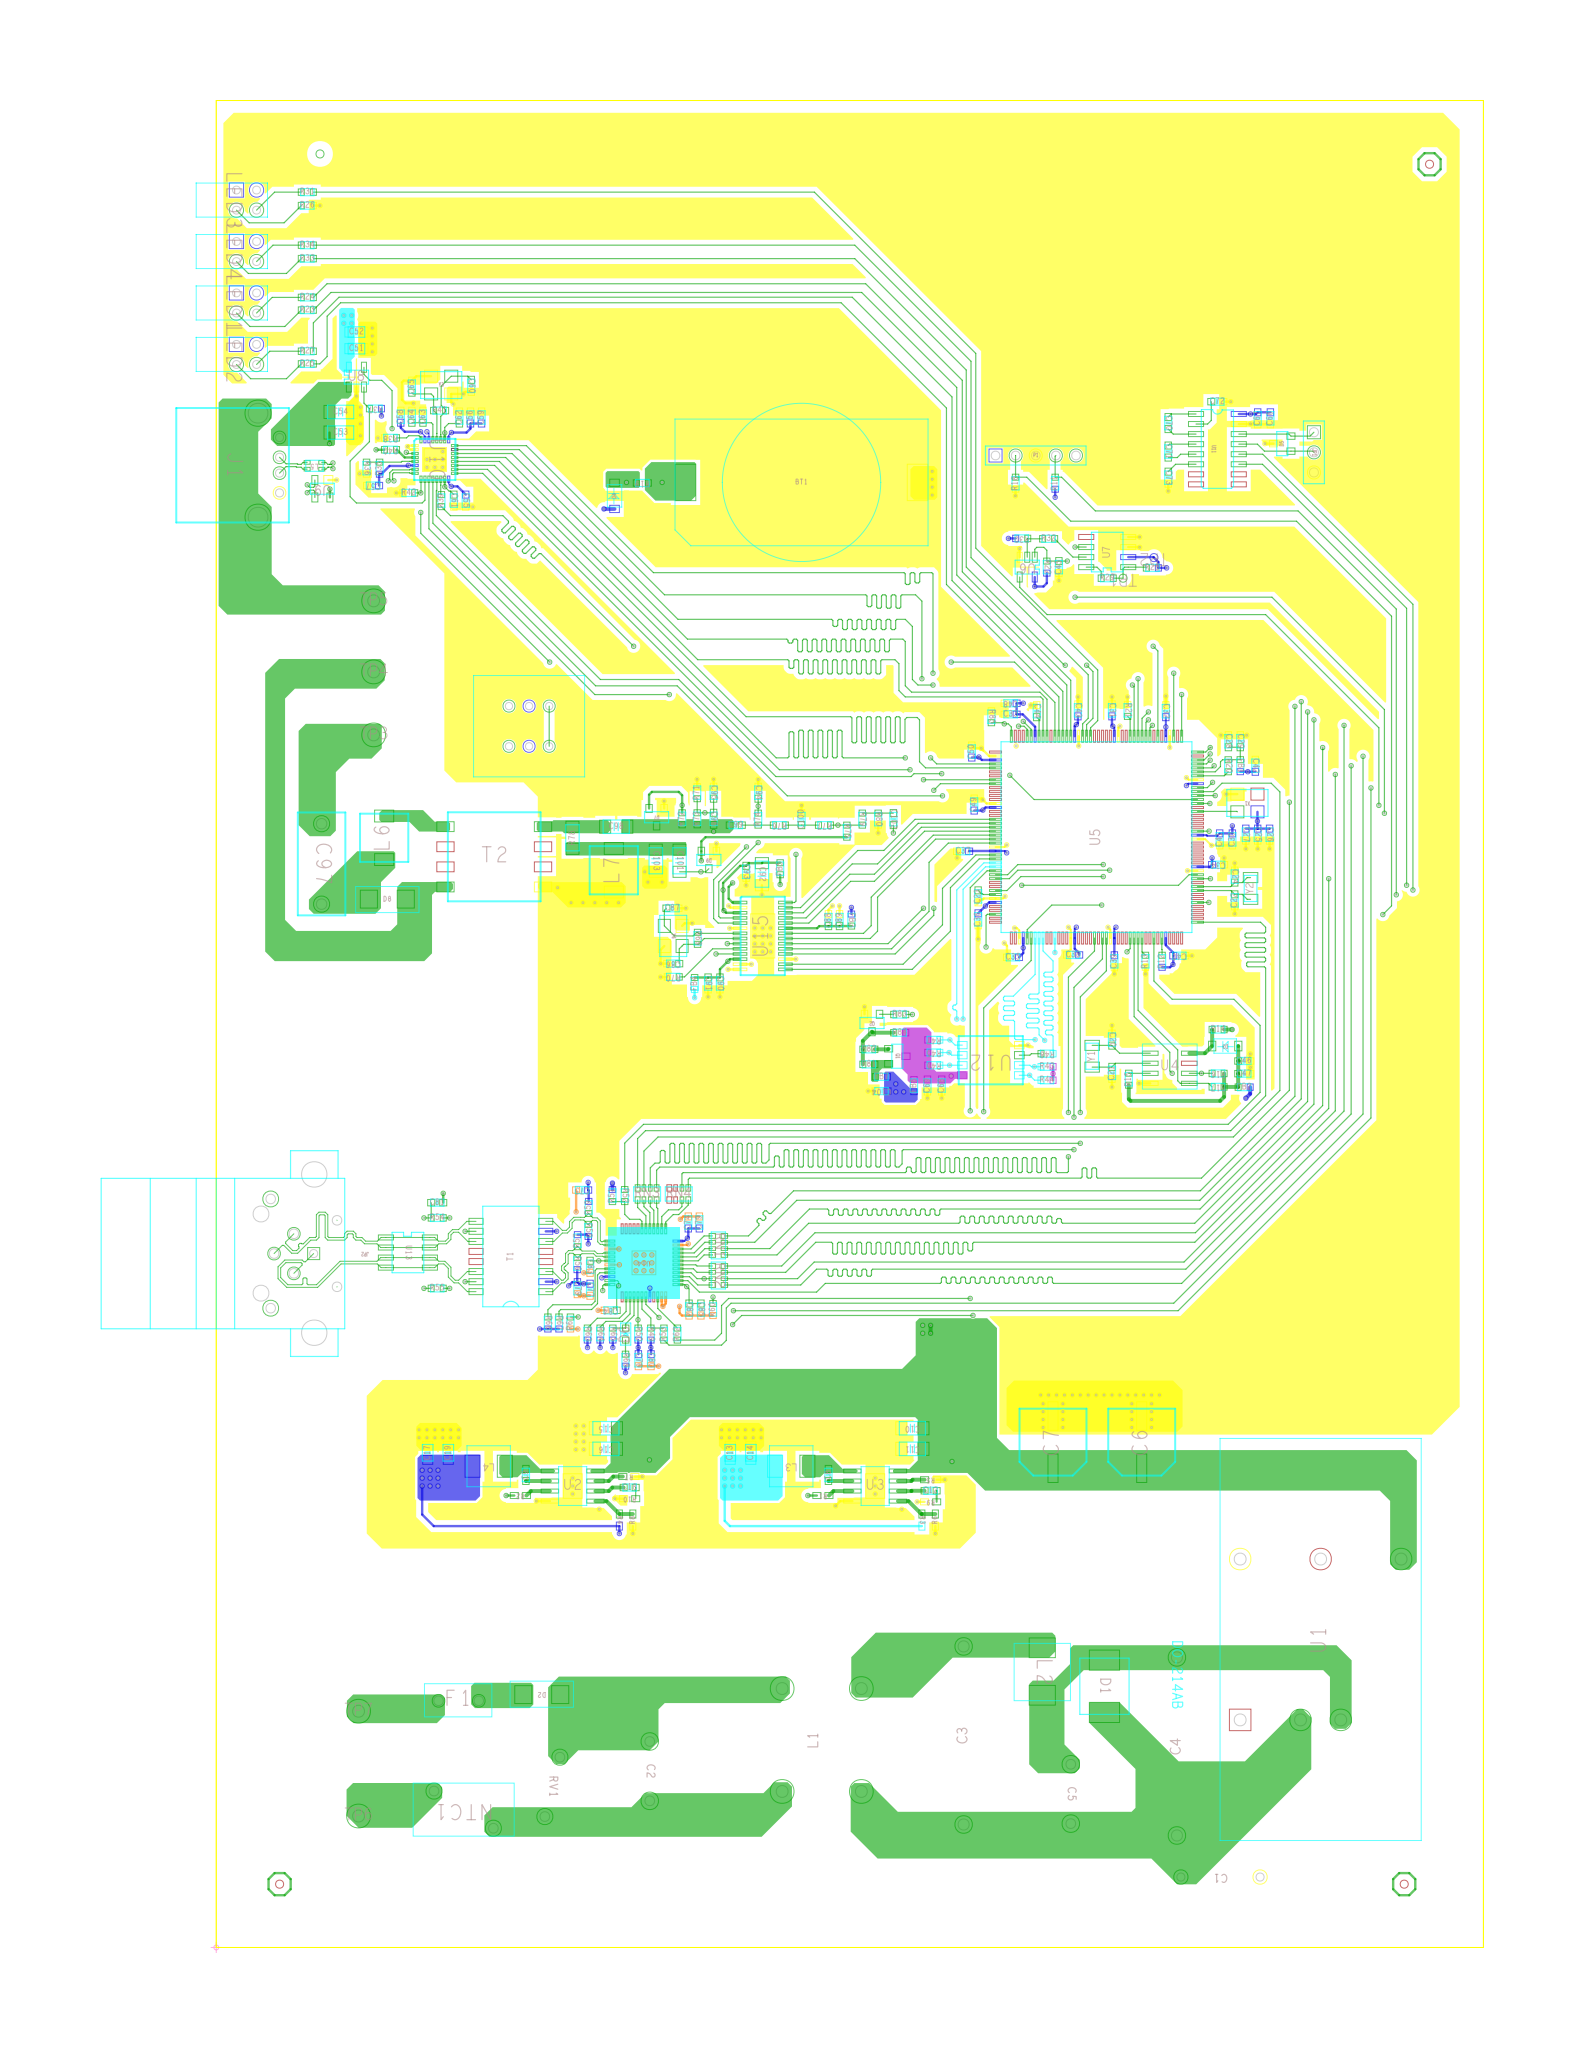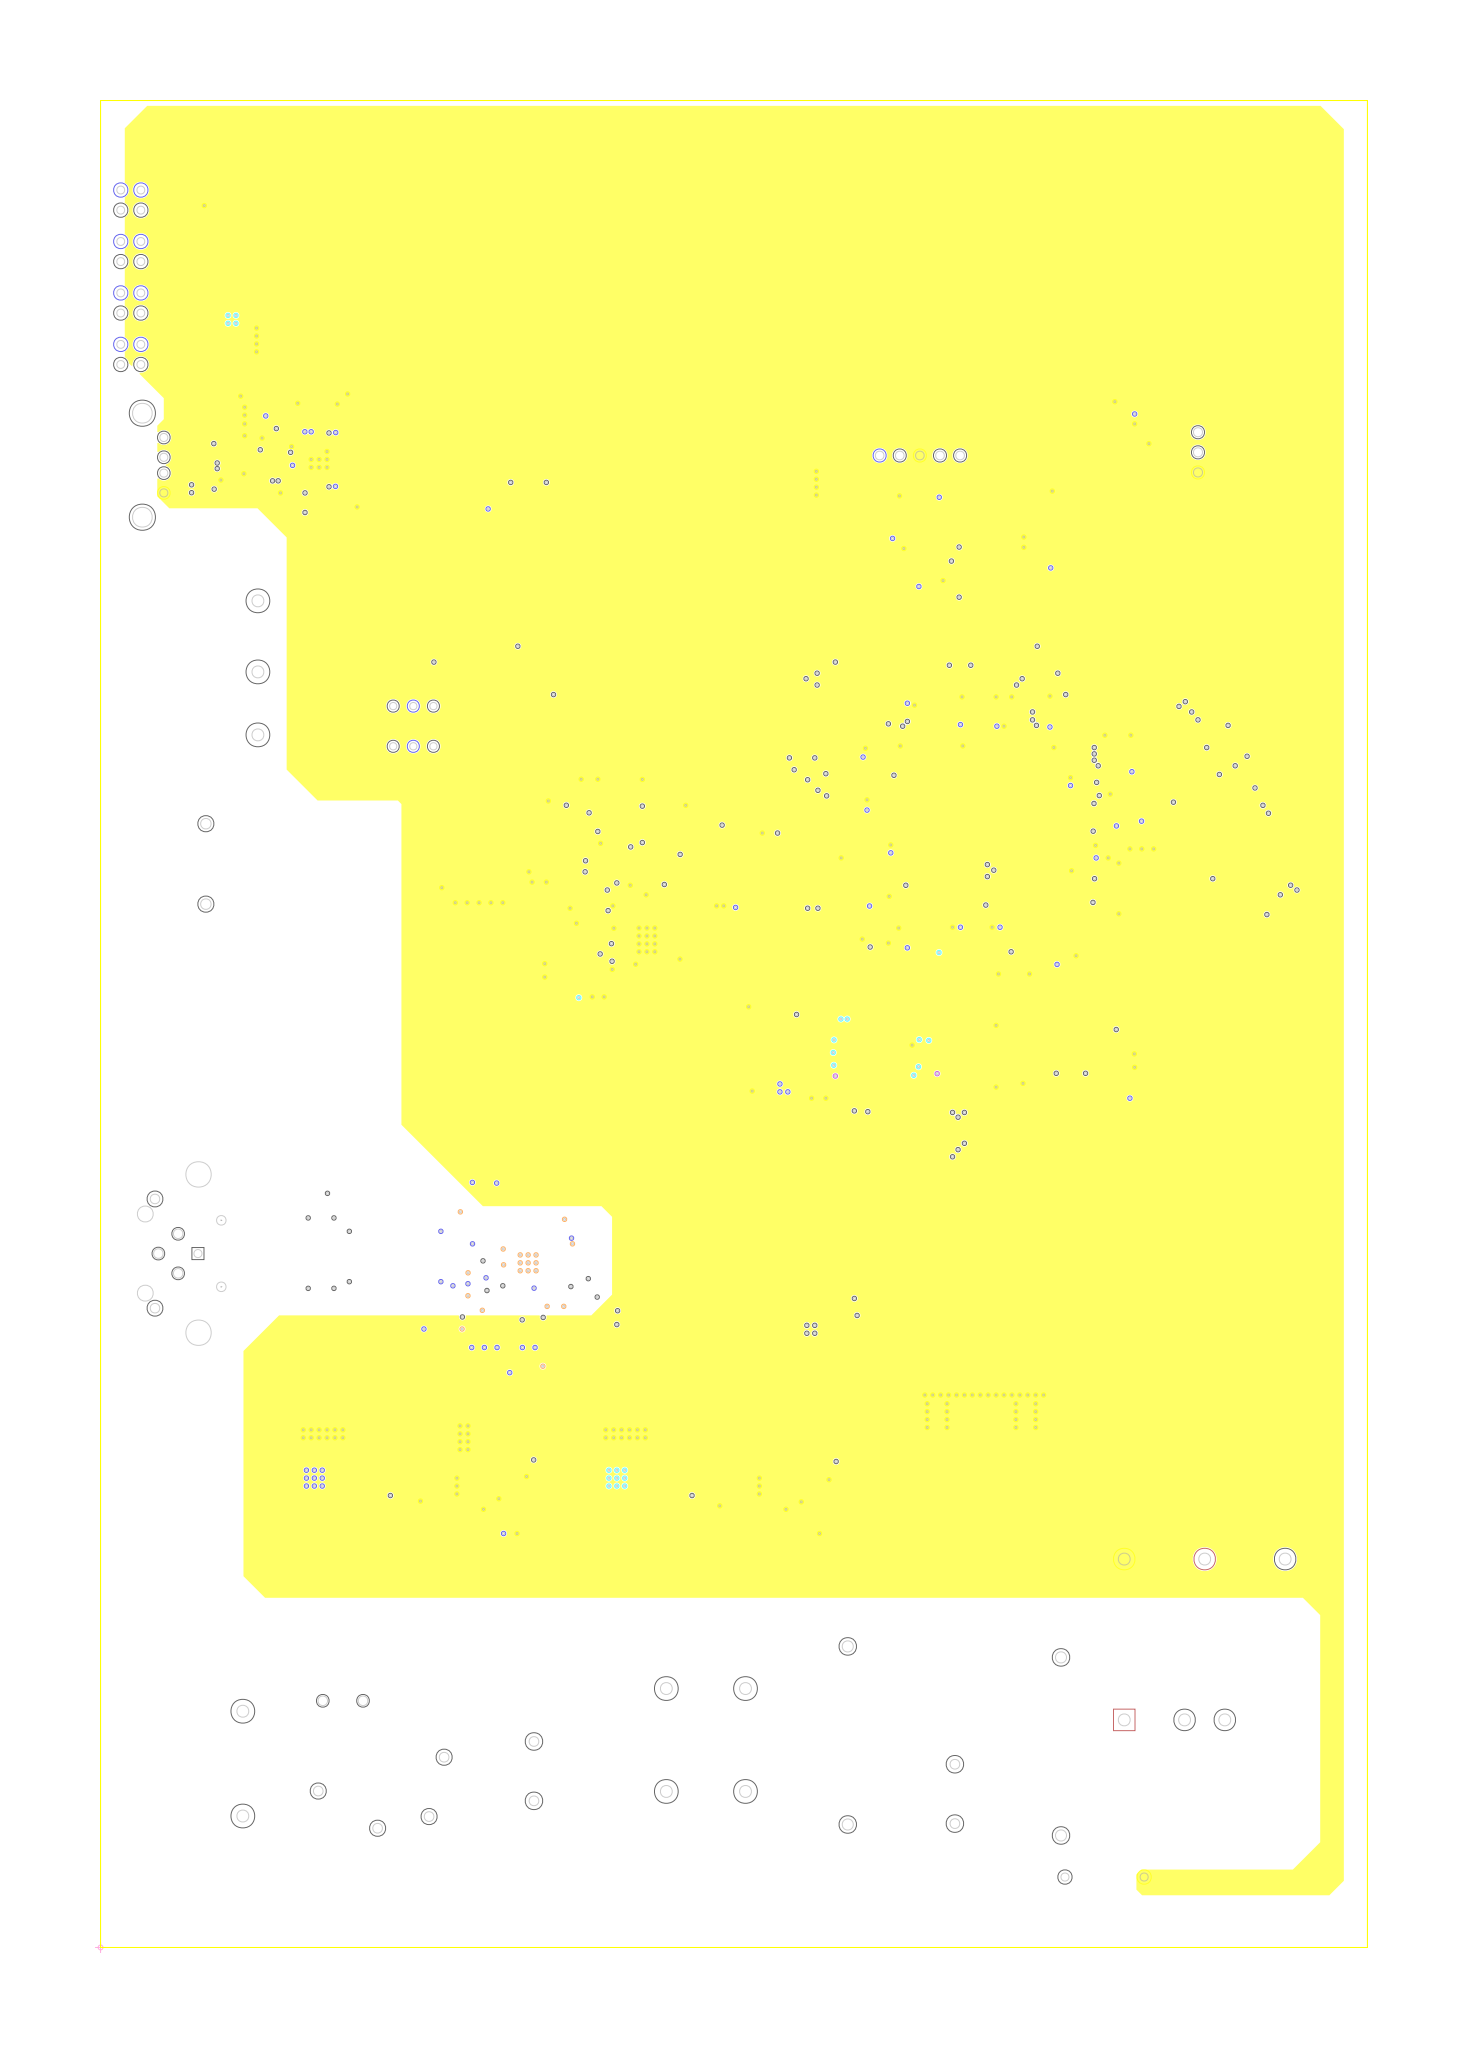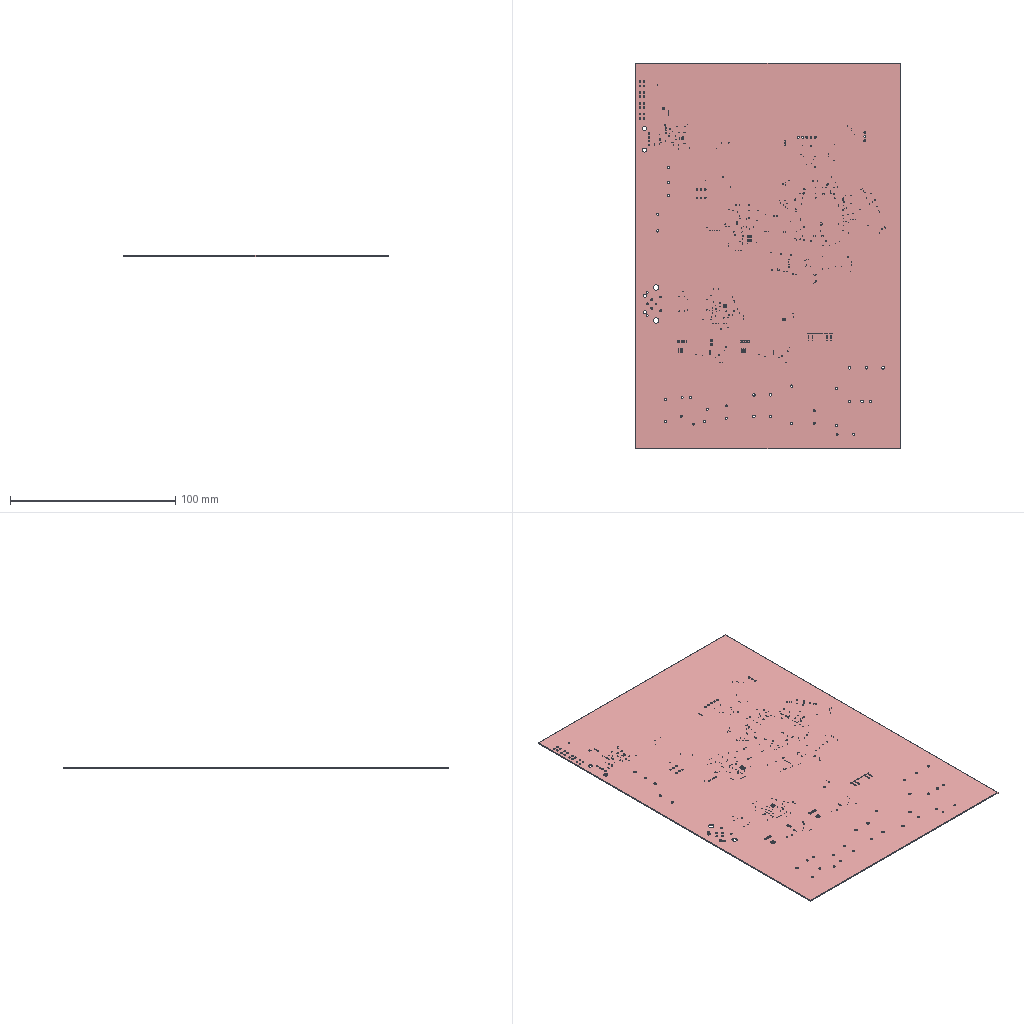Circuit board layout | Cadence Allegro | box 160 x 233.4 x 0.7 mm
Layer stack:
# Cadence Allegro layer stack of  (unit mm; from the constraint file cross-section; dielectric type: 0 not recorded (Allegro does not mark core vs prepreg), 3 surface material)
index,name,kind,layer,copper_thickness_mm,dielectric_type,dielectric_thickness_mm,dielectric_material,dielectric_constant
0,Top Surface,other,,,,,,
1,TOP,copper,TOP,0.0305,,,,
2,Dielectric1,dielectric,,,0,0.2032,FR-4,4.5
3,L2_GND,copper,L2_GND,0.0305,,,,
4,Dielectric2,dielectric,,,0,0.2032,FR-4,4.5
5,L3_PWR,copper,L3_PWR,0.0305,,,,
6,Dielectric3,dielectric,,,0,0.2032,FR-4,4.5
7,BOTTOM,copper,BOTTOM,0.0305,,,,
8,Bottom Surface,other,,,,,,
# drill layer pairs: low layer,high layer
drill_pair,TOP,BOTTOM
Part placement:
REFDES,COMP_VALUE,SYM_NAME,SYM_X,SYM_Y,SYM_ROTATE,SYM_MIRROR
BT1,,CON_BATTERY_CR2032,73.9,185.1,0.000,NO
C1,,CAP-TH_L10_0-W5_0-P10_00-D0_6,126.801,8.9,180.000,NO
C2,,CAP-TH_BD16_0-P7_50-D0_8-FD,54.737,22.276,270.000,NO
C3,,CAP-TH_L26_5-W10_0-P22_50-D1_4,94.369,26.788,90.000,NO
C4,,CAP-TH_L26_5-W10_0-P22_50-D1_4,121.3,25.4,90.000,NO
C5,,CAP-TH_BD16_0-P7_50-D0_8-FD,107.9,19.4,270.000,NO
C6,,CAP-SMD_BD8_0-L8_3-W8_3-LS9_0-FD_H10_2,116.854,63.846,90.000,NO
C7,,CAP-SMD_BD8_0-L8_3-W8_3-LS9_0-FD_H10_2,105.654,63.846,90.000,NO
C8,,0603-C,77.3,59.7,90.000,NO
C9,,0603-C,39.1,59.7,90.000,NO
C10,,1206-C,87.9,65.6,180.000,NO
C11,,1206-C,87.9,63,180.000,NO
C12,,0603-C,90.2,57.7,0.000,NO
C13,,0805-C,64.9,62.5,90.000,NO
C14,,0805-C,67.5,62.5,90.000,NO
C15,,1206-C,49.2,65.6,180.000,NO
C16,,1206-C,49.2,63,180.000,NO
C17,,0805-C,26.7,62.5,90.000,NO
C18,,0603-C,52.2,58.113,0.000,NO
C19,,0805-C,29.3,62.5,90.000,NO
C20,,0603-C,113.1,114.7,270.000,NO
C21,,0603-C,113.1,110.5,90.000,NO
C22,,0603-C,128.6,132.3,90.000,NO
C23,,0603-C,96.2,132.8,90.000,NO
C24,,0603-C,128.6,135.3,270.000,NO
C25,,0603-C,131.5,140.6,270.000,NO
C26,,0603-C,133,140.6,270.000,NO
C27,,0603-C,130,140.6,270.000,NO
C28,,0603-C,127.8,152.4,270.000,NO
C29,,0603-C,129.3,152.4,270.000,NO
C30,,0603-C,128.3,140,90.000,NO
C31,,0603-C,113.1,156.3,270.000,NO
C32,,0603-C,119.9,156.2,270.000,NO
C33,,0603-C,100.3,155.8,0.000,NO
C34,,0603-C,126.5,136.8,180.000,NO
C35,,0603-C,100.6,125.1,0.000,NO
C36,,0603-C,96.2,129.9,90.000,NO
C37,,0603-C,94.3,138.5,0.000,NO
C38,,0603-C,108.2,125.4,0.000,NO
C39,,0603-C,113.4,124.6,90.000,NO
C40,,0603-C,121.6,125.3,180.000,NO
C41,,0603-C,126.7,140,90.000,NO
C42,,0603-C,131.2,149.3,270.000,NO
C43,,0603-C,108.8,156.3,270.000,NO
C44,,0603-C,103.6,156.2,270.000,NO
C45,,0603-C,106.4,174.4,90.000,NO
C46,,0603-C,129.8,112,0.000,NO
C47,,0603-C,129.8,110.4,0.000,NO
C48,,0603-C,100.3,157.2,180.000,NO
C49,,0603-C,95.7,144.4,90.000,NO
C50,,0603-C,95.4,151.1,90.000,NO
C51,,0805-C,17.7,202,0.000,NO
C52,,0805-C,17.7,204.1,0.000,NO
C53,,1206-C,15.7,191.4,0.000,NO
C54,,1206-C,15.7,194,0.000,NO
C55,,0603-C,31.5,182.8,270.000,NO
C56,,0603-C,32.1,193.3,90.000,NO
C57,,0603-C,19.8,184.7,180.000,NO
C58,,0603-C,23.3,193.4,90.000,NO
C59,,0603-C,33.5,193.3,90.000,NO
C60,,0603-C,32.2,197.3,270.000,NO
C61,,0603-C,30,182.8,270.000,NO
C62,,0603-C,30.7,193.3,90.000,NO
C63,,0603-C,26.1,193.4,90.000,NO
C64,,0603-C,24.7,193.4,90.000,NO
C65,,0603-C,24.7,197.2,90.000,NO
C66,,0603-C,133.1,193.2,90.000,NO
C67,,0603-C,131.5,193.2,90.000,NO
C68,,0603-C,91.6,108.9,90.000,NO
C69,,0603-C,89.8,108.9,90.000,NO
C70,,0603-C,120.2,192.6,270.000,NO
C71,,0603-C,120.2,189,270.000,NO
C72,,0603-C,126.4,195.3,0.000,NO
C73,,0603-C,120.2,185.7,270.000,NO
C74,,0603-C,59.6,91.6,90.000,NO
C75,,0603-C,46.2,95.7,180.000,NO
C76,,0603-C,53.3,74.2,270.000,NO
C77,,0603-C,47.2,83.1,270.000,NO
C78,,0603-C,45.6,83.3,270.000,NO
C79,,0603-C,61,91.6,90.000,NO
C80,,0603-C,54.9,74.2,270.000,NO
C81,,0603-C,27.9,94.1,0.000,NO
C82,,0603-C,59.7,80.6,270.000,NO
C83,,0603-C,47.2,86,270.000,NO
C84,,0603-C,49.8,80.5,180.000,NO
C85,,0603-C,61.2,80.6,270.000,NO
C86,,0603-C,57.7,124.3,180.000,NO
C87,,0603-C,57.6,131.3,0.000,NO
C88,,0603-C,77.3,129.8,90.000,NO
C89,,0603-C,78.7,129.8,90.000,NO
C90,,0603-C,63.6,121.8,270.000,NO
C91,,0603-C,62.1,121.8,270.000,NO
C92,,1206-C,68.9,135.6,270.000,NO
C93,,0603-C,66.9,135.9,270.000,NO
C94,,0603-C,68.425,145.9,270.000,NO
C95,,0603-C,62.8,145.9,270.000,NO
C96,,0603-C,62.8,142.6,270.000,NO
C97,,CAP-TH_L13_0-W6_0-P10_00-D1_0,13.3,136.9,270.000,NO
C98,,1206-C,50.5,141.6,0.000,NO
C99,,0603-C,65.6,141.8,0.000,NO
C100,,0603-C,73.9,142.56,90.000,NO
C101,,1206-C,58.5,137.3,270.000,NO
C102,,0603-C,85.5,142.56,270.000,NO
C103,,1206-C,55.5,137.3,270.000,NO
C104,,0603-C,84,108.2,180.000,NO
D1,,SMC,112.15,33,270.000,NO
D2,,SMB,41.1,31.95,180.000,NO
D3,,SOD-123,127.4,113.89,180.000,NO
D4,,SOD-123,50.29,183.4,90.000,NO
D5,,SOT23-3-0_95-H1_11,134.6,190,90.000,NO
D6,,LED0603,51.7,77.5,90.000,NO
D7,,SOT23-3-0_95-H1_11,55.6,142.8,180.000,NO
D8,,SMB,21.6,132.45,0.000,NO
D9,,SOT23-3-0_95-H1_11,62.2,137.4,180.000,NO
F1,,FUSE-TH_L8_4-W4_0-P5_08-D0_6,30.607,31.166,0.000,NO
FB1,,0603-L,129.3,149.31,270.000,NO
FB2,,0603-L,129.79,108.7,0.000,NO
FB3,,0603-L,80.2,129.81,270.000,NO
FB4,,0603-L,60.4,121.79,90.000,NO
FB5,,0603-L,71.2,136.29,90.000,NO
FB6,,0603-L,88.1,108.89,90.000,NO
FB7,,0603-L,83.99,110,0.000,NO
J1,,USB-A-TH_USB-231-ARY,6.635,187.275,270.000,NO
JP1,,SIP3-2_54-MTP125,138.6,188.9,270.000,NO
JP2,,21033814412,9.8,87.67,180.000,NO
JP3,,6MD1S202M2QES,39.5,154.3,180.000,NO
L1,,FL2D-30-103,76.454,26.213,90.000,NO
L2,,IND-SMD_L7_9-W7_2,104.3,34.864,270.000,NO
L3,,SMD_LDPC0530RCP,72.6,60.8,180.000,NO
L4,,SMD_LDPC0530RCP,34.4,60.8,180.000,NO
L5,,L4-2_0X1_2X1_3-ACM2012,12.4,187.2,180.000,NO
L6,,IND-SMD_L6_0-W6_0_B82462A4473K000,21.2,140.2,90.000,NO
L7,,IND-SMD_L6_0-W6_0_B82462A4473K000,50.2,136.1,90.000,NO
LED1,,LED-TH_A694B2SYGS530-E2,3.82,207.77,270.000,NO
LED2,,LED-TH_A694B2SYGS530-E2,3.82,201.27,270.000,NO
LED3,,LED-TH_A694B2SYGS530-E2,3.82,220.77,270.000,NO
LED4,,LED-TH_A694B2SYGS530-E2,3.82,214.27,270.000,NO
NTC1,,RES-TH_L12_5-W6_5-P7_50-D1_2-S6_3,31.242,17.415,180.000,NO
P1,,5P2_54MM,103.475,188.5,0.000,NO
Q1,,SOT23-3-0_95-H1_11,86,112.6,270.000,NO
Q2,,SOT23-3-0_95-H1_11,82.8,116.8,180.000,NO
R1,,R0603,76.6,57.1,180.000,NO
R2,,R0603,38.4,57.1,180.000,NO
R3,,R0603,89.1,54,270.000,NO
R4,,R0603,50.9,54,270.000,NO
R5,,R0603,90.2,59.1,180.000,NO
R6,,R0603,90.8,54,90.000,NO
R7,,R0603,52.1,59.5,180.000,NO
R8,,R0603,52.6,54,90.000,NO
R9,,R0603,90.2,56.3,180.000,NO
R10,,R0603,52.2,56.7,180.000,NO
R11,,0603-R,105.925,185,90.000,NO
R12,,0603-R,119.425,124.6,90.000,NO
R13,,0603-R,117.325,124.6,90.000,NO
R14,,0603-R,126.5,115.975,0.000,NO
R15,,0603-R,115.225,109.7,90.000,NO
R16,,0603-R,126.5,110.425,180.000,NO
R17,,0603-R,126.5,108.725,180.000,NO
R18,,0603-R,100.925,185,90.000,NO
R19,,0603-R,53.8,185.025,180.000,NO
R20,,0603-R,127.775,149.3,270.000,NO
R21,,0603-R,115.075,156.3,270.000,NO
R22,,0603-R,104.875,174.4,270.000,NO
R23,,0603-R,11.5,206.875,0.000,NO
R24,,0603-R,11.5,208.475,0.000,NO
R25,,0603-R,11.5,200.075,0.000,NO
R26,,0603-R,11.5,220.075,0.000,NO
R27,,0603-R,11.5,201.675,0.000,NO
R28,,0603-R,118.2,174.3,0.000,NO
R29,,0603-R,112.5,173,0.000,NO
R30,,0603-R,101.7,178.025,180.000,NO
R31,,0603-R,11.5,221.775,0.000,NO
R32,,0603-R,105.1,177.975,0.000,NO
R33,,0603-R,11.5,213.375,0.000,NO
R34,,0603-R,11.5,215.075,0.000,NO
R35,,0603-R,20.625,186.9,90.000,NO
R36,,0603-R,18.975,186.9,270.000,NO
R37,,0603-R,20.1,194.425,180.000,NO
R38,,0603-R,22,190.725,180.000,NO
R39,,0603-R,28.425,182.8,90.000,NO
R40,,0603-R,22,189.225,180.000,NO
R41,,0603-R,28.2,194.175,0.000,NO
R42,,0603-R,24.3,183.775,0.000,NO
R43,,0603-R,104.9,111.275,0.000,NO
R44,,0603-R,104.9,109.575,0.000,NO
R45,,0603-R,90.6,113.065,180.000,NO
R46,,0603-R,90.6,111.465,180.000,NO
R47,,0603-R,90.6,114.665,180.000,NO
R48,,0603-R,104.9,112.925,180.000,NO
R49,,0603-R,54.875,77.5,270.000,NO
R50,,0603-R,53.275,77.5,270.000,NO
R51,,0603-R,50.025,95,90.000,NO
R52,,0603-R,51.575,95,270.000,NO
R53,,0603-R,56.525,77.5,90.000,NO
R54,,0603-R,27.9,92.175,0.000,NO
R55,,0603-R,27.9,83.275,0.000,NO
R56,,0603-R,45.575,86.4,270.000,NO
R57,,0603-R,45.625,89.3,90.000,NO
R58,,0603-R,46.975,90.6,270.000,NO
R59,,0603-R,47.025,93.5,90.000,NO
R60,,0603-R,62.725,80.6,90.000,NO
R61,,0603-R,44.725,78.9,90.000,NO
R62,,0603-R,58.225,77.5,90.000,NO
R63,,0603-R,46.875,77.5,270.000,NO
R64,,0603-R,48.475,77.5,270.000,NO
R65,,0603-R,50.075,77.5,270.000,NO
R66,,0603-R,41.875,78.9,270.000,NO
R67,,0603-R,43.275,78.9,270.000,NO
R68,,0603-R,51.675,74.2,270.000,NO
R69,,0603-R,60.775,127.5,270.000,NO
R70,,0603-R,57.7,122.625,180.000,NO
R71,,0603-R,60.725,145.9,90.000,NO
R72,,0603-R,58.825,142.6,90.000,NO
R73,,0603-R,60.725,142.6,90.000,NO
R74,,0603-R,68.425,142.56,90.000,NO
R75,,0603-R,79.625,141.04,270.000,NO
R76,,0603-R,71.1,141.8,180.000,NO
R77,,0603-R,76.8,141.8,180.000,NO
R78,,1206-R,44.975,140.2,90.000,NO
R79,,0603-R,81.575,142.56,270.000,NO
R80,,0603-R,83.575,142.56,270.000,NO
R81,,0603-R,82.4,111.575,0.000,NO
R82,,0603-R,82.4,113.475,0.000,NO
R83,,0603-R,86.3,117.875,0.000,NO
R84,,0603-R,86.3,115.575,0.000,NO
R85,,0603-R,97.875,155.5,270.000,NO
RN1,,RN0603,63.4,88.7,270.000,NO
RN2,,RN0603,63.4,84.9,270.000,NO
RN3,,RN0603,54.4,95.2,0.000,NO
RN4,,RN0603,58.4,95.2,0.000,NO
RV1,,RES-TH_L16_5-W4_2-P7_50-D1_2-S1_90,42.441,20.29,270.000,NO
T1,,TFM16-1_27-7_11-5_97,37.2,87.3,90.000,NO
T2,,T60403-K5024-X044_VAC,35.1,137.8,0.000,NO
TP1,,TP_SMD1MMCIRCLE,114.5,173,180.000,NO
TP2,,TP_SMD1MMCIRCLE,118.4,175.6,180.000,NO
TP3,,TP52_80,19.873,153.203,0.000,NO
TP4,,TP52_80,19.873,161.16,0.000,NO
TP5,,TP52_80,19.873,170.137,0.000,NO
TP6,,TP52_80,17.968,16.609,0.000,NO
TP7,,TP52_80,17.968,29.849,0.000,NO
U1,,PWRM-TH_5P-L50_8-W25_4-P5_08_URB1D24LMD-10WR3,139.446,38.913,90.000,NO
U2,,SMD_DDA,45,58.3,270.000,NO
U3,,SMD_DDA,83.2,58.3,270.000,NO
U4,,21-0041B_8,120.4,111.078,0.000,NO
U5,,LQFP176,111.144,140.285,90.000,NO
U6,,SOT-23-5-0_95-H1_45,102.4,174.4,180.000,NO
U7,,SOIC8-1_27-3_98-1_75,112.5,176.3,90.000,NO
U8,,SOT-23-5-0_95-H1_45,17.7,198.4,0.000,NO
U9,,SOT143-4-3_0X1_4-H1_15,13.4,184.3,180.000,NO
U10,,QFN-32_L5_0-W5_0-P0_50-BL-EP3_4,27.6,188.001,270.000,NO
U11,,SOIC16-1_27-5_4,126.413,189.3,270.000,NO
U12,,LGA-8_L8_0-W6_0-TL_MKDV4GIL-AS,97.8,112.1,180.000,NO
U13,,SOIC8-1_27-5_1X4_0-H1_75,24.2,87.8,270.000,NO
U14,,QFP_48,54,86.5,180.000,NO
U15,,HTSSOP-28_L9_7-W4_4-P0_65-LS6_4-BL-EP,69,127.8,90.000,NO
X1,,X4-5_0X3_2-SG5032,130.2,144.6,180.000,NO
Y1,,X2-3_2X1_5-FC-135R,110.6,112.6,90.000,NO
Y2,,X2-3_2X1_5-FC-135R,130.6,133.8,90.000,NO
Y3,,X4-5_0X3_2-SG5032,28.4,197.4,0.000,NO
Y4,,X4-5_0X3_2-SG5032,57.7,127.8,270.000,NO
Pad and via stacks:
# Allegro (Cadence) via spans and padstacks; design units: ("millimeters" 4 10000)
# via spans: padstack,start_layer,end_layer,net_example,count
# Allegro padstack definitions: name,start_layer,end_layer,drill,plating,holeType,type
MARK40-120-BOT,"ETCH/BOTTOM","ETCH/BOTTOM",0.0,"PLATED","none","smd"
MARK40-120,"ETCH/TOP","ETCH/TOP",0.0,"PLATED","none","smd"
ID-BOARD,"ETCH/TOP","ETCH/TOP",0.0,"PLATED","none","smd"
SMD55_65,"ETCH/TOP","ETCH/TOP",0.0,"PLATED","none","smd"
SMD35_32,"ETCH/TOP","ETCH/TOP",0.0,"PLATED","none","smd"
SMD40X30,"ETCH/TOP","ETCH/TOP",0.0,"PLATED","none","smd"
SMD25_20,"ETCH/TOP","ETCH/TOP",0.0,"PLATED","none","smd"
SMD45_50,"ETCH/TOP","ETCH/TOP",0.0,"PLATED","none","smd"
SMD100_150,"ETCH/TOP","ETCH/TOP",0.0,"PLATED","none","smd"
SMD_R1063X1299P0S20,"ETCH/TOP","ETCH/TOP",0.0,"PLATED","none","smd"
SMD32_40,"ETCH/TOP","ETCH/TOP",0.0,"PLATED","none","smd"
SMD30_32,"ETCH/TOP","ETCH/TOP",0.0,"PLATED","none","smd"
SMD40_50,"ETCH/TOP","ETCH/TOP",0.0,"PLATED","none","smd"
SMD98_130,"ETCH/TOP","ETCH/TOP",0.0,"NON_PLATED","none","smd"
RECT75X110,"ETCH/TOP","ETCH/TOP",0.0,"PLATED","none","smd"
SMD59_95,"ETCH/TOP","ETCH/TOP",0.0,"NON_PLATED","none","smd"
SMD30_70,"ETCH/TOP","ETCH/TOP",0.0,"NON_PLATED","none","smd"
SMD86_49,"ETCH/TOP","ETCH/TOP",0.0,"NON_PLATED","none","smd"
40SMD,"ETCH/TOP","ETCH/TOP",0.0,"PLATED","none","smd"
SMD25_75,"ETCH/TOP","ETCH/TOP",0.0,"PLATED","none","smd"
SMD36_48,"ETCH/TOP","ETCH/TOP",0.0,"PLATED","none","smd"
SMD13_68,"ETCH/TOP","ETCH/TOP",0.0,"NON_PLATED","none","smd"
SMD220_120,"ETCH/TOP","ETCH/TOP",0.0,"NON_PLATED","none","smd"
SMD05X22,"ETCH/TOP","ETCH/TOP",0.0,"PLATED","none","smd"
SMD31X24,"ETCH/TOP","ETCH/TOP",0.0,"PLATED","none","smd"
SMD25_50,"ETCH/TOP","ETCH/TOP",0.0,"PLATED","none","smd"
SMD65_60,"ETCH/TOP","ETCH/TOP",0.0,"PLATED","none","smd"
SMD1_3X1_1MM,"ETCH/TOP","ETCH/TOP",0.0,"PLATED","none","smd"
SMD46X26,"ETCH/TOP","ETCH/TOP",0.0,"PLATED","none","smd"
36X48,"ETCH/TOP","ETCH/TOP",0.0,"PLATED","none","smd"
SMD85_89,"ETCH/TOP","ETCH/TOP",0.0,"NON_PLATED","none","smd"
SMD30_18,"ETCH/TOP","ETCH/TOP",0.0,"PLATED","none","smd"
SMD32_11,"ETCH/TOP","ETCH/TOP",0.0,"NON_PLATED","none","smd"
SMD11_32,"ETCH/TOP","ETCH/TOP",0.0,"NON_PLATED","none","smd"
SMD107_107,"ETCH/TOP","ETCH/TOP",0.0,"NON_PLATED","none","smd"
SMD60_10,"ETCH/TOP","ETCH/TOP",0.0,"PLATED","none","smd"
SMD10_60,"ETCH/TOP","ETCH/TOP",0.0,"PLATED","none","smd"
SMD3R00SQMMSP,"ETCH/TOP","ETCH/TOP",0.0,"NON_PLATED","none","smd"
REC10X50,"ETCH/TOP","ETCH/TOP",0.0,"PLATED","none","smd"
SMD24_32,"ETCH/TOP","ETCH/TOP",0.0,"PLATED","none","smd"
SMD18_32,"ETCH/TOP","ETCH/TOP",0.0,"PLATED","none","smd"
SMD78_21,"ETCH/TOP","ETCH/TOP",0.0,"PLATED","none","smd"
SMD50_72,"ETCH/TOP","ETCH/TOP",0.0,"PLATED","none","smd"
SMD30_45,"ETCH/TOP","ETCH/TOP",0.0,"PLATED","none","smd"
SMD45_45,"ETCH/TOP","ETCH/TOP",0.0,"PLATED","none","smd"
SMD142_50,"ETCH/TOP","ETCH/TOP",0.0,"NON_PLATED","none","smd"
VIA10-GEN,"ETCH/TOP","ETCH/BOTTOM",0.254,"PLATED","circle_drill","through"
VIA10-BGA-FULL,"ETCH/TOP","ETCH/BOTTOM",0.254,"PLATED","circle_drill","through"
VIA12-GEN,"ETCH/TOP","ETCH/BOTTOM",0.3048,"PLATED","circle_drill","through"
VIA12-BGA-FULL,"ETCH/TOP","ETCH/BOTTOM",0.3048,"PLATED","circle_drill","through"
VIA16,"ETCH/TOP","ETCH/BOTTOM",0.4064,"PLATED","circle_drill","through"
VIA24,"ETCH/TOP","ETCH/BOTTOM",0.6096,"PLATED","circle_drill","through"
VIA8-BGA-FULL-NEW,"ETCH/TOP","ETCH/BOTTOM",0.2032,"PLATED","circle_drill","through"
BGA-TVIA10-32,"ETCH/TOP","ETCH/BOTTOM",0.254,"PLATED","circle_drill","through"
BGA-TVIA10-40,"ETCH/TOP","ETCH/BOTTOM",0.254,"PLATED","circle_drill","through"
BGA-TVIA12-32,"ETCH/TOP","ETCH/BOTTOM",0.3048,"PLATED","circle_drill","through"
TVIA16-32,"ETCH/TOP","ETCH/BOTTOM",0.4064,"PLATED","circle_drill","through"
TVIA16-40,"ETCH/TOP","ETCH/BOTTOM",0.4064,"PLATED","circle_drill","through"
TVIA10-32,"ETCH/TOP","ETCH/BOTTOM",0.254,"PLATED","circle_drill","through"
TVIA10-40,"ETCH/TOP","ETCH/BOTTOM",0.254,"PLATED","circle_drill","through"
TVIA12-32,"ETCH/TOP","ETCH/BOTTOM",0.3048,"PLATED","circle_drill","through"
TVIA12-40,"ETCH/TOP","ETCH/BOTTOM",0.3048,"PLATED","circle_drill","through"
PAD32CIR32U,"ETCH/TOP","ETCH/BOTTOM",0.8128,"NON_PLATED","circle_drill","through"
PAD80CIR80U,"ETCH/TOP","ETCH/BOTTOM",2.032,"NON_PLATED","circle_drill","through"
RE48_44X28D,"ETCH/TOP","ETCH/BOTTOM",0.7112,"PLATED","circle_drill","through"
RE44_60X28D,"ETCH/TOP","ETCH/BOTTOM",0.7112,"PLATED","circle_drill","through"
PAD71CIR40D,"ETCH/TOP","ETCH/BOTTOM",1.016,"PLATED","circle_drill","through"
PAD87CIR48D,"ETCH/TOP","ETCH/BOTTOM",1.219,"PLATED","circle_drill","through"
PAD87CIR55D,"ETCH/TOP","ETCH/BOTTOM",1.397,"PLATED","circle_drill","through"
PAD60CIR40D,"ETCH/TOP","ETCH/BOTTOM",1.2,"PLATED","circle_drill","through"
PAD65SQ45D,"ETCH/TOP","ETCH/BOTTOM",1.143,"PLATED","circle_drill","through"
PAD65CIR45D,"ETCH/TOP","ETCH/BOTTOM",1.143,"PLATED","circle_drill","through"
PAD71CIR39D,"ETCH/TOP","ETCH/BOTTOM",0.9906,"PLATED","circle_drill","through"
PAD71SQ39D,"ETCH/TOP","ETCH/BOTTOM",0.9906,"PLATED","circle_drill","through"
PAD80CIR48D,"ETCH/TOP","ETCH/BOTTOM",1.219,"PLATED","circle_drill","through"
PAD65SQ43D,"ETCH/TOP","ETCH/BOTTOM",1.092,"PLATED","circle_drill","through"
PAD65CIR43D,"ETCH/TOP","ETCH/BOTTOM",1.092,"PLATED","circle_drill","through"
PAD107CIR59D,"ETCH/TOP","ETCH/BOTTOM",1.499,"PLATED","circle_drill","through"
PAD107SQ59D,"ETCH/TOP","ETCH/BOTTOM",1.499,"PLATED","circle_drill","through"
VIA,"ETCH/TOP","ETCH/BOTTOM",0.3302,"PLATED","circle_drill","through"
PAD98CIR130D,"ETCH/TOP","ETCH/BOTTOM",2.489,"PLATED","circle_drill","through"
PAD40CIR69D,"ETCH/TOP","ETCH/BOTTOM",1.016,"PLATED","circle_drill","through"
PAD118CIR59D,"ETCH/TOP","ETCH/BOTTOM",1.499,"PLATED","circle_drill","through"
PAD150CIR130D,"ETCH/TOP","ETCH/BOTTOM",3.302,"PLATED","circle_drill","through"
PAD60SQ40D,"ETCH/TOP","ETCH/BOTTOM",1.016,"PLATED","circle_drill","through"
PAD52CIR80D,"ETCH/TOP","ETCH/BOTTOM",1.321,"PLATED","circle_drill","through"
PAD36CIR60D,"ETCH/TOP","ETCH/BOTTOM",0.9144,"PLATED","circle_drill","through"
THC2P0D1P2,"ETCH/TOP","ETCH/BOTTOM",1.2,"PLATED","circle_drill","through"
THC3P0D1P5,"ETCH/TOP","ETCH/BOTTOM",1.5,"PLATED","circle_drill","through"
HOLE3P3,"ETCH/TOP","ETCH/BOTTOM",3.2,"NON_PLATED","circle_drill","through"
HOLE2P0,"ETCH/TOP","ETCH/BOTTOM",2.0,"NON_PLATED","circle_drill","through"
HOLE1P2,"ETCH/TOP","ETCH/BOTTOM",1.2,"NON_PLATED","circle_drill","through"
Design rules, without the lines most boards share, first 13 of 36 lines:
# Cadence Allegro design rules of  (from the Constraint Manager export constraints.dcfx, design unit mm; typed fields in mm)
# columns: name | kind | enabled | priority | scope1 | scope2 | descriptor | typed fields (field=value)
# Allegro precedence (priority 1 wins): 1 Region class-to-class, 2 Region class, 3 Region, 4 class-to-class, 5 DiffPair/Bus/NetGroup override, 6 NetClass, 7 constraint set (CSet) default
# per-layer values are written LAYER=value in the descriptor and LAYER:mm in the typed field; a maximum of 0 means no limit set
# --- net classes (and buses / net groups) ---
DIFF100 | NetClass | enabled | 6 | ETH_RXD, ETH_TXD, ETH_RX, ETH_TX | All | Net Class (PhysicalCSet=DIFF100) (members: 4 DiffPair) overrides: (DIFFP_PHASE_TOL=0.2 mm) | physicalcset=DIFF100 diffp_phase_tol=0.2mm
PWR | NetClass | enabled | 6 | VDC, VDD, VDD_I2C3, VDD_3V3, GND, GND_EARTH, +5V0, +12V0, DGND, +12V0_ST7540, USB_POWER, VBUS, BAT, PA_OUT, TF_3V3 | All | Net Class (PhysicalCSet=PWR) (members: 15 Net) | physicalcset=PWR
DIFF90 | NetClass | enabled | 6 | D, DIFF_USB2 | All | Net Class (PhysicalCSet=DIFF90) (members: 2 DiffPair) overrides: (DIFFP_PHASE_TOL=0.2 mm) | physicalcset=DIFF90 diffp_phase_tol=0.2mm
# --- track widths, neck and differential-pair gap (physical constraint sets) ---
PWR | PhysicalCSet | enabled | 7 | NetClass(1): PWR | All | Physical Constraint (Min Line Width=0.3048mm) (Max Line Width=0mm) (Min Neck Width=0.127mm) (Max Neck Length=254mm) (DiffPair Primary Gap=0mm) (DiffPair Neck Gap=0mm) (DiffPair Min Space=0mm) (DiffPair Coupled +Tol=0mm) (DiffPair Coupled -Tol=0mm) (Min BB Via Stagger=0.127mm) (Max BB Via Stagger=0mm) (T-junctions=ANYWHERE) (Pad-pad direct connect=ALL_ALLOWED) (Allowed vias=VIA10-BGA-FULL, VIA8-BGA-FULL-NEW) | min_line_width=0.3048 min_neck_width=0.127 min_bvia_stagger=0.127 max_bvia_stagger=0 ts_allowed=ANYWHERE diffp_primary_gap=0 diffp_neck_gap=0 max_line_width=0 maximum_neck_length=254 pad_pad_direct_connect=ALL_ALLOWED allow_on_etch_subclass=TRUE diffp_coupled_plus=0 diffp_coupled_minus=0 diffp_min_space=0 vias=VIA10-BGA-FULL,VIA8-BGA-FULL-NEW
DIFF90 | PhysicalCSet | enabled | 7 | NetClass(1): DIFF90 | All | Physical Constraint (Min Line Width=0.1549mm) (Max Line Width=0mm) (Min Neck Width=0.1016mm) (Max Neck Length=0mm) (DiffPair Primary Gap=0.2032mm) (DiffPair Neck Gap=0mm) (DiffPair Min Space=0.1016mm) (DiffPair Coupled +Tol=0mm) (DiffPair Coupled -Tol=0mm) (Min BB Via Stagger=0.127mm) (Max BB Via Stagger=0mm) (T-junctions=ANYWHERE) (Pad-pad direct connect=ALL_ALLOWED) (Allowed vias=VIA10-BGA-FULL, VIA8-BGA-FULL-NEW) | min_line_width=0.1549 min_neck_width=0.1016 min_bvia_stagger=0.127 max_bvia_stagger=0 ts_allowed=ANYWHERE diffp_primary_gap=0.2032 diffp_neck_gap=0 max_line_width=0 maximum_neck_length=0 pad_pad_direct_connect=ALL_ALLOWED allow_on_etch_subclass=TRUE diffp_coupled_plus=0 diffp_coupled_minus=0 diffp_min_space=0.1016 vias=VIA10-BGA-FULL,VIA8-BGA-FULL-NEW
DIFF100 | PhysicalCSet | enabled | 7 | NetClass(1): DIFF100 | All | Physical Constraint (Min Line Width=0.1295mm) (Max Line Width=0mm) (Min Neck Width=0.1016mm) (Max Neck Length=254mm) (DiffPair Primary Gap=0.2032mm) (DiffPair Neck Gap=0mm) (DiffPair Min Space=0.1016mm) (DiffPair Coupled +Tol=0mm) (DiffPair Coupled -Tol=0mm) (Min BB Via Stagger=0.127mm) (Max BB Via Stagger=0mm) (T-junctions=ANYWHERE) (Pad-pad direct connect=ALL_ALLOWED) (Allowed vias=VIA10-BGA-FULL, VIA8-BGA-FULL-NEW) | min_line_width=0.1295 min_neck_width=0.1016 min_bvia_stagger=0.127 max_bvia_stagger=0 ts_allowed=ANYWHERE diffp_primary_gap=0.2032 diffp_neck_gap=0 max_line_width=0 maximum_neck_length=254 pad_pad_direct_connect=ALL_ALLOWED allow_on_etch_subclass=TRUE diffp_coupled_plus=0 diffp_coupled_minus=0 diffp_min_space=0.1016 vias=VIA10-BGA-FULL,VIA8-BGA-FULL-NEW
DEFAULT | PhysicalCSet | enabled | 7 | Design default; Net(1): BAT | All | Physical Constraint (Min Line Width=0.1524mm) (Max Line Width=0mm) (Min Neck Width=0.1016mm) (Max Neck Length=254mm) (DiffPair Primary Gap=0mm) (DiffPair Neck Gap=0mm) (DiffPair Min Space=0mm) (DiffPair Coupled +Tol=0mm) (DiffPair Coupled -Tol=0mm) (Min BB Via Stagger=0.127mm) (Max BB Via Stagger=0mm) (T-junctions=ANYWHERE) (Pad-pad direct connect=ALL_ALLOWED) (Allowed vias=VIA10-BGA-FULL, VIA8-BGA-FULL-NEW) | min_line_width=0.1524 min_neck_width=0.1016 min_bvia_stagger=0.127 max_bvia_stagger=0 ts_allowed=ANYWHERE diffp_primary_gap=0 diffp_neck_gap=0 max_line_width=0 maximum_neck_length=254 pad_pad_direct_connect=ALL_ALLOWED allow_on_etch_subclass=TRUE diffp_coupled_plus=0 diffp_coupled_minus=0 diffp_min_space=0 vias=VIA10-BGA-FULL,VIA8-BGA-FULL-NEW